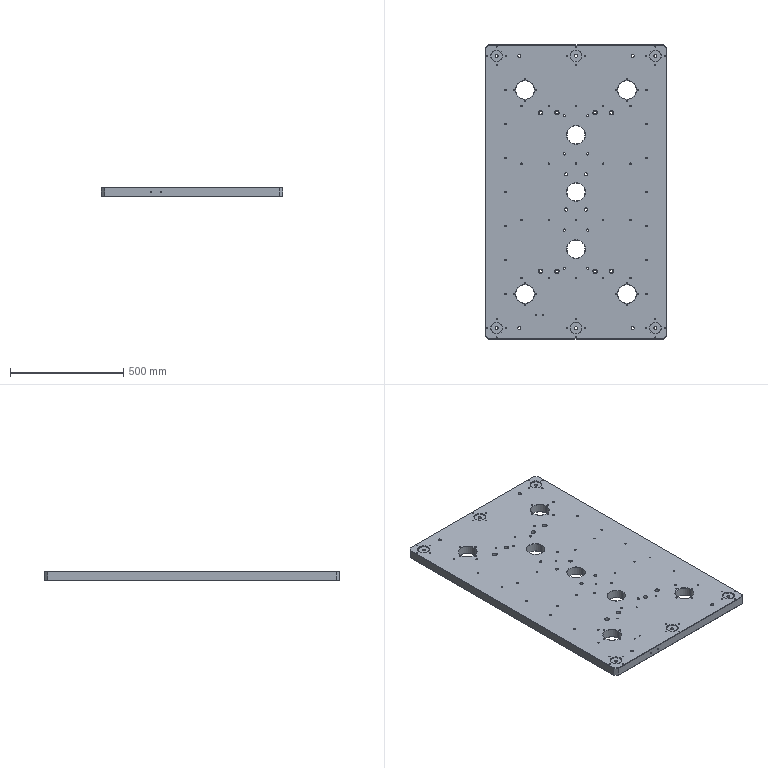Part | STEP file | TJ-DHQM-003-001 | 1 solid | 504 faces | box 800 x 1300 x 40 mm | volume 39783539 mm3 | cylinder 342 | cone 116 | plane 46 | commonest cylinder face diameters 6.8 x104 5 x68 3.3 x44 13.5 x28 20 x28 10.2 x16